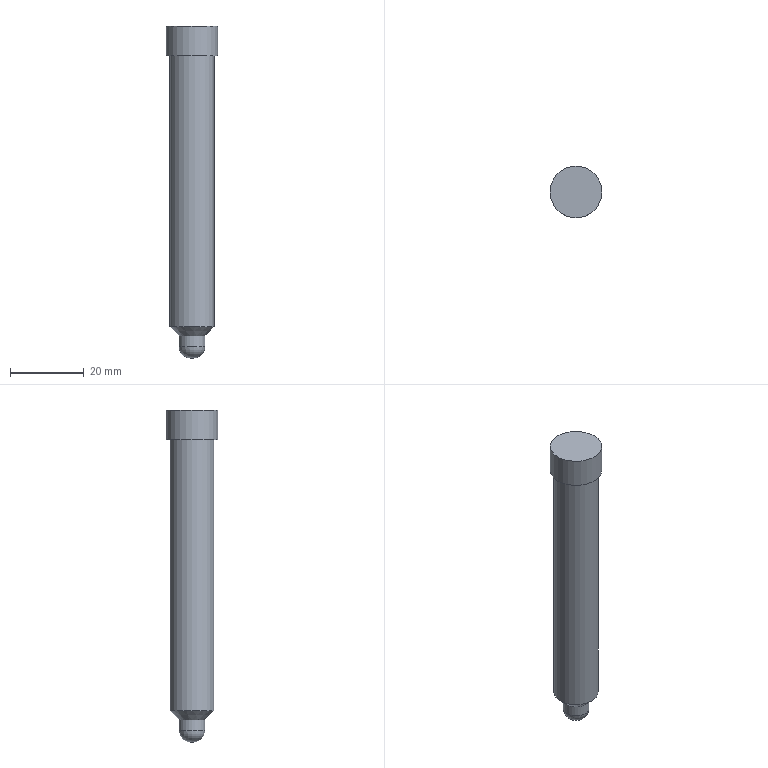Part | NX | features solid 2 | 1 solid | 8 faces | box 14 x 14 x 90 mm | volume 9922 mm3 | cylinder 3 | plane 3 | torus 1 | cone 1 | commonest cylinder face diameters 7 x1 12 x1 14 x1
STEP:
#1=CARTESIAN_POINT('',(2465.097,-906.796,864.216));
#2=VERTEX_POINT('',#1);
#3=CARTESIAN_POINT('',(2459.097,-906.796,864.216));
#4=DIRECTION('',(0.,0.,-1.));
#5=DIRECTION('',(1.,0.,0.));
#6=AXIS2_PLACEMENT_3D('',#3,#4,#5);
#7=CIRCLE('',#6,6.);
#8=EDGE_CURVE('',#2,#2,#7,.T.);
#9=ORIENTED_EDGE('',*,*,#8,.F.);
#10=EDGE_LOOP('',(#9));
#11=FACE_BOUND('',#10,.T.);
#12=CARTESIAN_POINT('',(2465.097,-906.796,937.716));
#13=VERTEX_POINT('',#12);
#14=CARTESIAN_POINT('',(2459.097,-906.796,937.716));
#15=DIRECTION('',(0.,0.,-1.));
#16=DIRECTION('',(1.,0.,0.));
#17=AXIS2_PLACEMENT_3D('',#14,#15,#16);
#18=CIRCLE('',#17,6.);
#19=EDGE_CURVE('',#13,#13,#18,.F.);
#20=ORIENTED_EDGE('',*,*,#19,.F.);
#21=EDGE_LOOP('',(#20));
#22=FACE_BOUND('',#21,.T.);
#23=CARTESIAN_POINT('',(2459.097,-906.796,940.716));
#24=DIRECTION('',(0.,0.,-1.));
#25=DIRECTION('',(-1.,0.,0.));
#26=AXIS2_PLACEMENT_3D('',#23,#24,#25);
#27=CYLINDRICAL_SURFACE('',#26,6.);
#28=ADVANCED_FACE('',(#11,#22),#27,.T.);
#29=CARTESIAN_POINT('',(2466.097,-906.796,945.716));
#30=VERTEX_POINT('',#29);
#31=CARTESIAN_POINT('',(2459.097,-906.796,945.716));
#32=DIRECTION('',(0.,0.,-1.));
#33=DIRECTION('',(1.,0.,0.));
#34=AXIS2_PLACEMENT_3D('',#31,#32,#33);
#35=CIRCLE('',#34,7.);
#36=EDGE_CURVE('',#30,#30,#35,.T.);
#37=ORIENTED_EDGE('',*,*,#36,.F.);
#38=EDGE_LOOP('',(#37));
#39=FACE_BOUND('',#38,.T.);
#40=CARTESIAN_POINT('',(2261.069,-963.469,945.716));
#41=DIRECTION('',(0.,0.,1.));
#42=DIRECTION('',(-1.,0.,0.));
#43=AXIS2_PLACEMENT_3D('',#40,#41,#42);
#44=PLANE('',#43);
#45=ADVANCED_FACE('',(#39),#44,.T.);
#46=CARTESIAN_POINT('',(2466.097,-906.796,937.716));
#47=VERTEX_POINT('',#46);
#48=CARTESIAN_POINT('',(2459.097,-906.796,937.716));
#49=DIRECTION('',(0.,0.,1.));
#50=DIRECTION('',(1.,0.,0.));
#51=AXIS2_PLACEMENT_3D('',#48,#49,#50);
#52=CIRCLE('',#51,7.);
#53=EDGE_CURVE('',#47,#47,#52,.F.);
#54=ORIENTED_EDGE('',*,*,#53,.F.);
#55=EDGE_LOOP('',(#54));
#56=FACE_BOUND('',#55,.T.);
#57=ORIENTED_EDGE('',*,*,#36,.T.);
#58=EDGE_LOOP('',(#57));
#59=FACE_BOUND('',#58,.T.);
#60=CARTESIAN_POINT('',(2459.097,-906.796,950.716));
#61=DIRECTION('',(0.,0.,-1.));
#62=DIRECTION('',(-1.,0.,0.));
#63=AXIS2_PLACEMENT_3D('',#60,#61,#62);
#64=CYLINDRICAL_SURFACE('',#63,7.);
#65=ADVANCED_FACE('',(#56,#59),#64,.T.);
#66=ORIENTED_EDGE('',*,*,#19,.T.);
#67=EDGE_LOOP('',(#66));
#68=FACE_BOUND('',#67,.T.);
#69=ORIENTED_EDGE('',*,*,#53,.T.);
#70=EDGE_LOOP('',(#69));
#71=FACE_BOUND('',#70,.T.);
#72=CARTESIAN_POINT('',(2459.097,-906.796,937.716));
#73=DIRECTION('',(0.,0.,1.));
#74=DIRECTION('',(1.,0.,0.));
#75=AXIS2_PLACEMENT_3D('',#72,#73,#74);
#76=PLANE('',#75);
#77=ADVANCED_FACE('',(#68,#71),#76,.F.);
#78=CARTESIAN_POINT('',(2458.597,-906.796,855.716));
#79=VERTEX_POINT('',#78);
#80=CARTESIAN_POINT('',(2459.097,-906.796,855.716));
#81=DIRECTION('',(0.,0.,1.));
#82=DIRECTION('',(-1.,0.,0.));
#83=AXIS2_PLACEMENT_3D('',#80,#81,#82);
#84=CIRCLE('',#83,0.5);
#85=EDGE_CURVE('',#79,#79,#84,.T.);
#86=ORIENTED_EDGE('',*,*,#85,.F.);
#87=EDGE_LOOP('',(#86));
#88=FACE_BOUND('',#87,.T.);
#89=CARTESIAN_POINT('',(2459.097,-906.796,855.716));
#90=DIRECTION('',(0.,0.,-1.));
#91=DIRECTION('',(-1.,0.,0.));
#92=AXIS2_PLACEMENT_3D('',#89,#90,#91);
#93=PLANE('',#92);
#94=ADVANCED_FACE('',(#88),#93,.T.);
#95=CARTESIAN_POINT('',(2455.597,-906.796,858.716));
#96=VERTEX_POINT('',#95);
#97=CARTESIAN_POINT('',(2459.097,-906.796,858.716));
#98=DIRECTION('',(0.,0.,1.));
#99=DIRECTION('',(-1.,0.,0.));
#100=AXIS2_PLACEMENT_3D('',#97,#98,#99);
#101=CIRCLE('',#100,3.5);
#102=EDGE_CURVE('',#96,#96,#101,.F.);
#103=ORIENTED_EDGE('',*,*,#102,.F.);
#104=EDGE_LOOP('',(#103));
#105=FACE_BOUND('',#104,.T.);
#106=CARTESIAN_POINT('',(2462.597,-906.796,861.716));
#107=VERTEX_POINT('',#106);
#108=CARTESIAN_POINT('',(2459.097,-906.796,861.716));
#109=DIRECTION('',(0.,0.,-1.));
#110=DIRECTION('',(1.,0.,0.));
#111=AXIS2_PLACEMENT_3D('',#108,#109,#110);
#112=CIRCLE('',#111,3.5);
#113=EDGE_CURVE('',#107,#107,#112,.F.);
#114=ORIENTED_EDGE('',*,*,#113,.F.);
#115=EDGE_LOOP('',(#114));
#116=FACE_BOUND('',#115,.T.);
#117=CARTESIAN_POINT('',(2459.097,-906.796,860.716));
#118=DIRECTION('',(0.,0.,-1.));
#119=DIRECTION('',(1.,0.,0.));
#120=AXIS2_PLACEMENT_3D('',#117,#118,#119);
#121=CYLINDRICAL_SURFACE('',#120,3.5);
#122=ADVANCED_FACE('',(#105,#116),#121,.T.);
#123=ORIENTED_EDGE('',*,*,#85,.T.);
#124=EDGE_LOOP('',(#123));
#125=FACE_BOUND('',#124,.T.);
#126=ORIENTED_EDGE('',*,*,#102,.T.);
#127=EDGE_LOOP('',(#126));
#128=FACE_BOUND('',#127,.T.);
#129=CARTESIAN_POINT('',(2459.097,-906.796,858.716));
#130=DIRECTION('',(0.,0.,-1.));
#131=DIRECTION('',(-1.,0.,0.));
#132=AXIS2_PLACEMENT_3D('',#129,#130,#131);
#133=DEGENERATE_TOROIDAL_SURFACE('',#132,0.5,3.,.T.);
#134=ADVANCED_FACE('',(#125,#128),#133,.T.);
#135=ORIENTED_EDGE('',*,*,#113,.T.);
#136=EDGE_LOOP('',(#135));
#137=FACE_BOUND('',#136,.T.);
#138=ORIENTED_EDGE('',*,*,#8,.T.);
#139=EDGE_LOOP('',(#138));
#140=FACE_BOUND('',#139,.T.);
#141=CARTESIAN_POINT('',(2459.097,-906.796,864.216));
#142=DIRECTION('',(0.,0.,1.));
#143=DIRECTION('',(1.,0.,0.));
#144=AXIS2_PLACEMENT_3D('',#141,#142,#143);
#145=CONICAL_SURFACE('',#144,6.,0.7854);
#146=ADVANCED_FACE('',(#137,#140),#145,.T.);
#147=CLOSED_SHELL('',(#28,#45,#65,#77,#94,#122,#134,#146));
#148=MANIFOLD_SOLID_BREP('',#147);
#149=(LENGTH_UNIT()NAMED_UNIT(*)SI_UNIT(.MILLI.,.METRE.));
#150=UNCERTAINTY_MEASURE_WITH_UNIT(LENGTH_MEASURE(0.00001),#149,'','');
#151=(NAMED_UNIT(*)PLANE_ANGLE_UNIT()SI_UNIT($,.RADIAN.));
#152=(NAMED_UNIT(*)SI_UNIT($,.STERADIAN.)SOLID_ANGLE_UNIT());
#153=(GEOMETRIC_REPRESENTATION_CONTEXT(3)GLOBAL_UNCERTAINTY_ASSIGNED_CONTEXT((#150))GLOBAL_UNIT_ASSIGNED_CONTEXT((#149,#151,#152))REPRESENTATION_CONTEXT('',''));
#154=ADVANCED_BREP_SHAPE_REPRESENTATION('',(#148),#153);